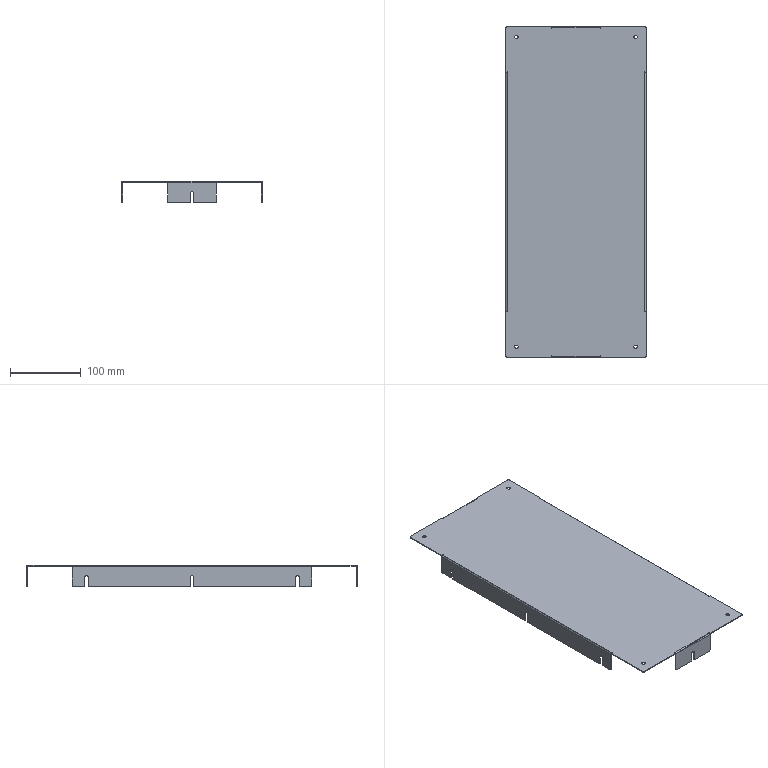Part | STEP file | 1 solid | 128 faces | box 199 x 469 x 30 mm | volume 138914 mm3 | plane 86 | cylinder 42 | commonest cylinder face diameters 4.5 x14 4 x12 5 x8 1.2 x4 3.6 x4